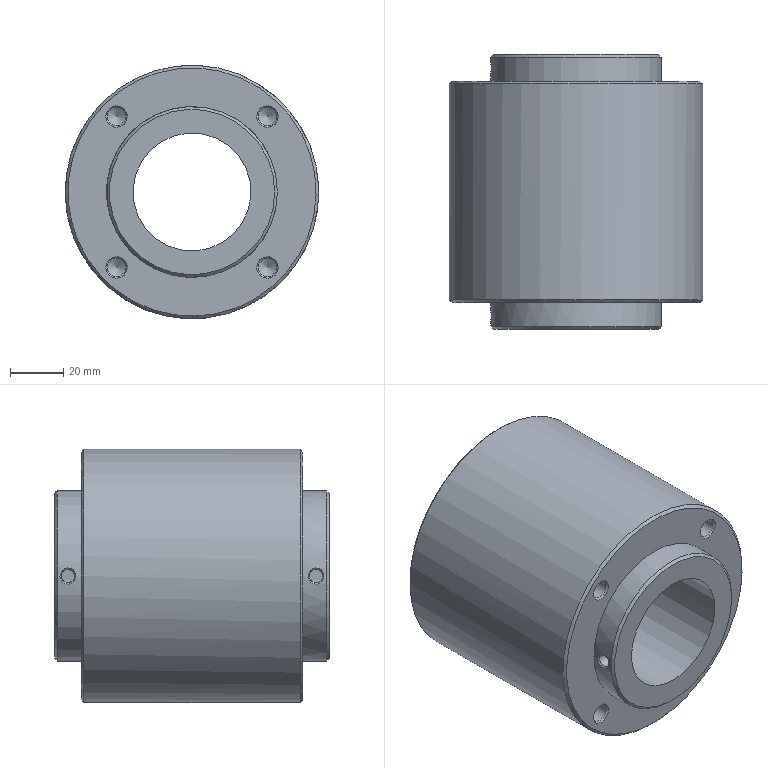Part | STEP file | YBQDJ-FLJ-2 | 1 solid | 42 faces | box 95 x 103 x 95 mm | volume 482469 mm3 | cone 20 | cylinder 14 | plane 4 | spline 4 | commonest cylinder face diameters 6.8 x8 5 x2 64 x2 44.2 x1 95 x1